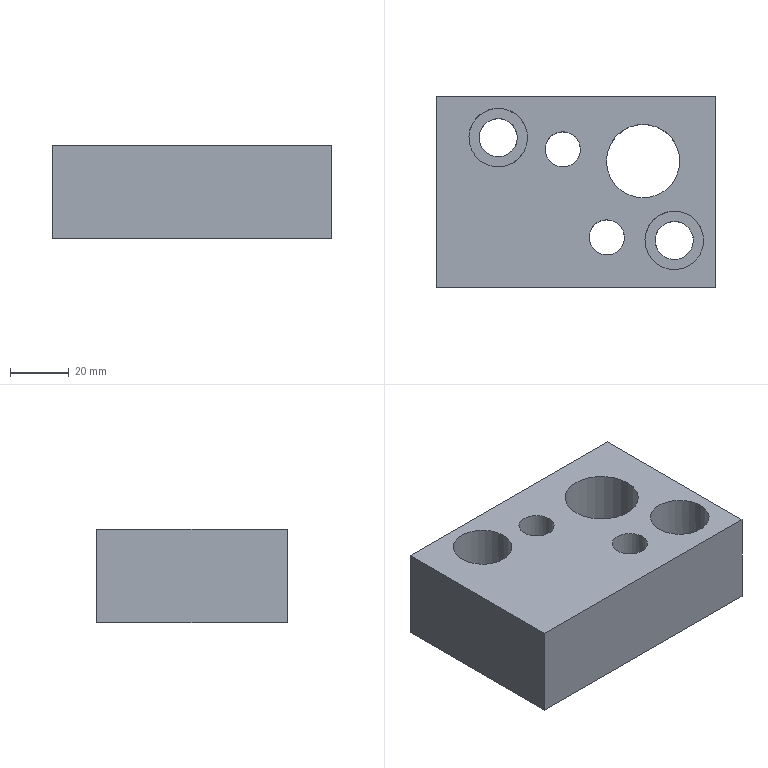Part | STEP file | gslz 2016.10.28-13_id1334_x_t | 1 solid | 17 faces | box 95 x 65 x 32 mm | volume 157873 mm3 | plane 9 | cylinder 8 | commonest cylinder face diameters 12 x2 13 x2 20 x2 25 x1 32 x1
STEP:
#1=CARTESIAN_POINT('',(0.,0.,0.));
#2=DIRECTION('',(0.,0.,1.));
#3=DIRECTION('',(1.,0.,0.));
#4=AXIS2_PLACEMENT_3D('',#1,#2,#3);
#5=CARTESIAN_POINT('',(-1412.127,66.996,-26.4));
#6=VERTEX_POINT('',#5);
#7=CARTESIAN_POINT('',(-1424.627,66.996,-26.4));
#8=DIRECTION('',(0.,0.,1.));
#9=DIRECTION('',(1.,0.,0.));
#10=AXIS2_PLACEMENT_3D('',#7,#8,#9);
#11=CIRCLE('',#10,12.5);
#12=CARTESIAN_POINT('',(-1424.627,66.996,-26.4));
#13=DIRECTION('',(0.,0.,1.));
#14=DIRECTION('',(1.,0.,0.));
#15=AXIS2_PLACEMENT_3D('',#12,#13,#14);
#16=PLANE('',#15);
#17=CARTESIAN_POINT('',(0.,0.));
#18=DIRECTION('',(1.,0.));
#19=AXIS2_PLACEMENT_2D('',#17,#18);
#20=CIRCLE('',#19,12.5);
#21=(GEOMETRIC_REPRESENTATION_CONTEXT(2)PARAMETRIC_REPRESENTATION_CONTEXT()REPRESENTATION_CONTEXT('',''));
#22=DEFINITIONAL_REPRESENTATION('',(#20),#21);
#23=PCURVE('',#16,#22);
#24=CARTESIAN_POINT('',(-1424.627,66.996,-84.));
#25=DIRECTION('',(0.,0.,1.));
#26=DIRECTION('',(1.,0.,0.));
#27=AXIS2_PLACEMENT_3D('',#24,#25,#26);
#28=CYLINDRICAL_SURFACE('',#27,12.5);
#29=CARTESIAN_POINT('',(0.,57.6));
#30=DIRECTION('',(1.,0.));
#31=VECTOR('',#30,1.);
#32=LINE('',#29,#31);
#33=(GEOMETRIC_REPRESENTATION_CONTEXT(2)PARAMETRIC_REPRESENTATION_CONTEXT()REPRESENTATION_CONTEXT('',''));
#34=DEFINITIONAL_REPRESENTATION('',(#32),#33);
#35=PCURVE('',#28,#34);
#36=SURFACE_CURVE('',#11,(#23,#35),.PCURVE_S1.);
#37=EDGE_CURVE('',#6,#6,#36,.T.);
#38=ORIENTED_EDGE('',*,*,#37,.T.);
#39=EDGE_LOOP('',(#38));
#40=FACE_BOUND('',#39,.T.);
#41=CARTESIAN_POINT('',(-1408.627,66.996,-26.4));
#42=VERTEX_POINT('',#41);
#43=CARTESIAN_POINT('',(-1424.627,66.996,-26.4));
#44=DIRECTION('',(0.,0.,-1.));
#45=DIRECTION('',(1.,0.,0.));
#46=AXIS2_PLACEMENT_3D('',#43,#44,#45);
#47=CIRCLE('',#46,16.);
#48=CARTESIAN_POINT('',(16.,0.));
#49=CARTESIAN_POINT('',(16.,-27.713));
#50=CARTESIAN_POINT('',(-8.,-13.856));
#51=CARTESIAN_POINT('',(-32.,0.));
#52=CARTESIAN_POINT('',(-8.,13.856));
#53=CARTESIAN_POINT('',(16.,27.713));
#54=CARTESIAN_POINT('',(16.,0.));
#55=(BOUNDED_CURVE()B_SPLINE_CURVE(2,(#48,#49,#50,#51,#52,#53,#54),.UNSPECIFIED.,.T.,.F.)B_SPLINE_CURVE_WITH_KNOTS((1,2,2,2,2,1),(-2.094,0.,2.094,4.189,6.283,8.378),.UNSPECIFIED.)CURVE()GEOMETRIC_REPRESENTATION_ITEM()RATIONAL_B_SPLINE_CURVE((1.,0.5,1.,0.5,1.,0.5,1.))REPRESENTATION_ITEM(''));
#56=(GEOMETRIC_REPRESENTATION_CONTEXT(2)PARAMETRIC_REPRESENTATION_CONTEXT()REPRESENTATION_CONTEXT('',''));
#57=DEFINITIONAL_REPRESENTATION('',(#55),#56);
#58=PCURVE('',#16,#57);
#59=CARTESIAN_POINT('',(-1424.627,66.996,-29.7));
#60=DIRECTION('',(0.,0.,-1.));
#61=DIRECTION('',(-1.,0.,0.));
#62=AXIS2_PLACEMENT_3D('',#59,#60,#61);
#63=CYLINDRICAL_SURFACE('',#62,16.);
#64=CARTESIAN_POINT('',(3.142,-3.3));
#65=DIRECTION('',(1.,0.));
#66=VECTOR('',#65,1.);
#67=LINE('',#64,#66);
#68=(GEOMETRIC_REPRESENTATION_CONTEXT(2)PARAMETRIC_REPRESENTATION_CONTEXT()REPRESENTATION_CONTEXT('',''));
#69=DEFINITIONAL_REPRESENTATION('',(#67),#68);
#70=PCURVE('',#63,#69);
#71=SURFACE_CURVE('',#47,(#58,#70),.PCURVE_S1.);
#72=EDGE_CURVE('',#42,#42,#71,.T.);
#73=ORIENTED_EDGE('',*,*,#72,.T.);
#74=EDGE_LOOP('',(#73));
#75=FACE_BOUND('',#74,.T.);
#76=ADVANCED_FACE('',(#40,#75),#16,.F.);
#77=CARTESIAN_POINT('',(-1400.,24.,0.));
#78=VERTEX_POINT('',#77);
#79=CARTESIAN_POINT('',(-1400.,89.,0.));
#80=VERTEX_POINT('',#79);
#81=CARTESIAN_POINT('',(-1400.,30.,0.));
#82=DIRECTION('',(0.,1.,0.));
#83=VECTOR('',#82,1.);
#84=LINE('',#81,#83);
#85=CARTESIAN_POINT('',(-1400.,30.,-35.));
#86=DIRECTION('',(1.,0.,0.));
#87=DIRECTION('',(0.,1.,0.));
#88=AXIS2_PLACEMENT_3D('',#85,#86,#87);
#89=PLANE('',#88);
#90=CARTESIAN_POINT('',(0.,35.));
#91=DIRECTION('',(1.,0.));
#92=VECTOR('',#91,1.);
#93=LINE('',#90,#92);
#94=(GEOMETRIC_REPRESENTATION_CONTEXT(2)PARAMETRIC_REPRESENTATION_CONTEXT()REPRESENTATION_CONTEXT('',''));
#95=DEFINITIONAL_REPRESENTATION('',(#93),#94);
#96=PCURVE('',#89,#95);
#97=CARTESIAN_POINT('',(-1374.,128.728,0.));
#98=DIRECTION('',(0.,0.,1.));
#99=DIRECTION('',(1.,0.,0.));
#100=AXIS2_PLACEMENT_3D('',#97,#98,#99);
#101=PLANE('',#100);
#102=CARTESIAN_POINT('',(-26.,-98.728));
#103=DIRECTION('',(0.,1.));
#104=VECTOR('',#103,1.);
#105=LINE('',#102,#104);
#106=(GEOMETRIC_REPRESENTATION_CONTEXT(2)PARAMETRIC_REPRESENTATION_CONTEXT()REPRESENTATION_CONTEXT('',''));
#107=DEFINITIONAL_REPRESENTATION('',(#105),#106);
#108=PCURVE('',#101,#107);
#109=SURFACE_CURVE('',#84,(#96,#108),.PCURVE_S1.);
#110=EDGE_CURVE('',#78,#80,#109,.T.);
#111=ORIENTED_EDGE('',*,*,#110,.F.);
#112=CARTESIAN_POINT('',(-1400.,24.,-32.));
#113=VERTEX_POINT('',#112);
#114=CARTESIAN_POINT('',(-1400.,24.,-35.));
#115=DIRECTION('',(0.,0.,1.));
#116=VECTOR('',#115,1.);
#117=LINE('',#114,#116);
#118=CARTESIAN_POINT('',(-6.,0.));
#119=DIRECTION('',(0.,1.));
#120=VECTOR('',#119,1.);
#121=LINE('',#118,#120);
#122=(GEOMETRIC_REPRESENTATION_CONTEXT(2)PARAMETRIC_REPRESENTATION_CONTEXT()REPRESENTATION_CONTEXT('',''));
#123=DEFINITIONAL_REPRESENTATION('',(#121),#122);
#124=PCURVE('',#89,#123);
#125=CARTESIAN_POINT('',(-1490.,24.,-35.));
#126=DIRECTION('',(0.,-1.,0.));
#127=DIRECTION('',(1.,0.,0.));
#128=AXIS2_PLACEMENT_3D('',#125,#126,#127);
#129=PLANE('',#128);
#130=CARTESIAN_POINT('',(90.,0.));
#131=DIRECTION('',(0.,1.));
#132=VECTOR('',#131,1.);
#133=LINE('',#130,#132);
#134=(GEOMETRIC_REPRESENTATION_CONTEXT(2)PARAMETRIC_REPRESENTATION_CONTEXT()REPRESENTATION_CONTEXT('',''));
#135=DEFINITIONAL_REPRESENTATION('',(#133),#134);
#136=PCURVE('',#129,#135);
#137=SURFACE_CURVE('',#117,(#124,#136),.PCURVE_S1.);
#138=EDGE_CURVE('',#113,#78,#137,.T.);
#139=ORIENTED_EDGE('',*,*,#138,.F.);
#140=CARTESIAN_POINT('',(-1400.,89.,-32.));
#141=VERTEX_POINT('',#140);
#142=CARTESIAN_POINT('',(-1400.,30.,-32.));
#143=DIRECTION('',(0.,1.,0.));
#144=VECTOR('',#143,1.);
#145=LINE('',#142,#144);
#146=CARTESIAN_POINT('',(0.,3.));
#147=DIRECTION('',(1.,0.));
#148=VECTOR('',#147,1.);
#149=LINE('',#146,#148);
#150=(GEOMETRIC_REPRESENTATION_CONTEXT(2)PARAMETRIC_REPRESENTATION_CONTEXT()REPRESENTATION_CONTEXT('',''));
#151=DEFINITIONAL_REPRESENTATION('',(#149),#150);
#152=PCURVE('',#89,#151);
#153=CARTESIAN_POINT('',(-1374.,128.728,-32.));
#154=DIRECTION('',(0.,0.,1.));
#155=DIRECTION('',(1.,0.,0.));
#156=AXIS2_PLACEMENT_3D('',#153,#154,#155);
#157=PLANE('',#156);
#158=CARTESIAN_POINT('',(-26.,-98.728));
#159=DIRECTION('',(0.,1.));
#160=VECTOR('',#159,1.);
#161=LINE('',#158,#160);
#162=(GEOMETRIC_REPRESENTATION_CONTEXT(2)PARAMETRIC_REPRESENTATION_CONTEXT()REPRESENTATION_CONTEXT('',''));
#163=DEFINITIONAL_REPRESENTATION('',(#161),#162);
#164=PCURVE('',#157,#163);
#165=SURFACE_CURVE('',#145,(#152,#164),.PCURVE_S1.);
#166=EDGE_CURVE('',#113,#141,#165,.T.);
#167=ORIENTED_EDGE('',*,*,#166,.T.);
#168=CARTESIAN_POINT('',(-1400.,89.,-35.));
#169=DIRECTION('',(0.,0.,-1.));
#170=VECTOR('',#169,1.);
#171=LINE('',#168,#170);
#172=CARTESIAN_POINT('',(59.,0.));
#173=DIRECTION('',(0.,-1.));
#174=VECTOR('',#173,1.);
#175=LINE('',#172,#174);
#176=(GEOMETRIC_REPRESENTATION_CONTEXT(2)PARAMETRIC_REPRESENTATION_CONTEXT()REPRESENTATION_CONTEXT('',''));
#177=DEFINITIONAL_REPRESENTATION('',(#175),#176);
#178=PCURVE('',#89,#177);
#179=CARTESIAN_POINT('',(-1445.,89.,-17.5));
#180=DIRECTION('',(0.,-1.,0.));
#181=DIRECTION('',(0.,0.,-1.));
#182=AXIS2_PLACEMENT_3D('',#179,#180,#181);
#183=PLANE('',#182);
#184=CARTESIAN_POINT('',(17.5,45.));
#185=DIRECTION('',(1.,0.));
#186=VECTOR('',#185,1.);
#187=LINE('',#184,#186);
#188=(GEOMETRIC_REPRESENTATION_CONTEXT(2)PARAMETRIC_REPRESENTATION_CONTEXT()REPRESENTATION_CONTEXT('',''));
#189=DEFINITIONAL_REPRESENTATION('',(#187),#188);
#190=PCURVE('',#183,#189);
#191=SURFACE_CURVE('',#171,(#178,#190),.PCURVE_S1.);
#192=EDGE_CURVE('',#80,#141,#191,.T.);
#193=ORIENTED_EDGE('',*,*,#192,.F.);
#194=EDGE_LOOP('',(#111,#139,#167,#193));
#195=FACE_BOUND('',#194,.T.);
#196=ADVANCED_FACE('',(#195),#89,.T.);
#197=CARTESIAN_POINT('',(-1495.,24.,0.));
#198=VERTEX_POINT('',#197);
#199=CARTESIAN_POINT('',(-1490.,24.,0.));
#200=DIRECTION('',(1.,0.,0.));
#201=VECTOR('',#200,1.);
#202=LINE('',#199,#201);
#203=CARTESIAN_POINT('',(0.,35.));
#204=DIRECTION('',(1.,0.));
#205=VECTOR('',#204,1.);
#206=LINE('',#203,#205);
#207=(GEOMETRIC_REPRESENTATION_CONTEXT(2)PARAMETRIC_REPRESENTATION_CONTEXT()REPRESENTATION_CONTEXT('',''));
#208=DEFINITIONAL_REPRESENTATION('',(#206),#207);
#209=PCURVE('',#129,#208);
#210=CARTESIAN_POINT('',(-116.,-104.728));
#211=DIRECTION('',(1.,0.));
#212=VECTOR('',#211,1.);
#213=LINE('',#210,#212);
#214=(GEOMETRIC_REPRESENTATION_CONTEXT(2)PARAMETRIC_REPRESENTATION_CONTEXT()REPRESENTATION_CONTEXT('',''));
#215=DEFINITIONAL_REPRESENTATION('',(#213),#214);
#216=PCURVE('',#101,#215);
#217=SURFACE_CURVE('',#202,(#209,#216),.PCURVE_S1.);
#218=EDGE_CURVE('',#198,#78,#217,.T.);
#219=ORIENTED_EDGE('',*,*,#218,.F.);
#220=CARTESIAN_POINT('',(-1495.,24.,-32.));
#221=VERTEX_POINT('',#220);
#222=CARTESIAN_POINT('',(-1495.,24.,-35.));
#223=DIRECTION('',(0.,0.,1.));
#224=VECTOR('',#223,1.);
#225=LINE('',#222,#224);
#226=CARTESIAN_POINT('',(-5.,0.));
#227=DIRECTION('',(0.,1.));
#228=VECTOR('',#227,1.);
#229=LINE('',#226,#228);
#230=(GEOMETRIC_REPRESENTATION_CONTEXT(2)PARAMETRIC_REPRESENTATION_CONTEXT()REPRESENTATION_CONTEXT('',''));
#231=DEFINITIONAL_REPRESENTATION('',(#229),#230);
#232=PCURVE('',#129,#231);
#233=CARTESIAN_POINT('',(-1495.,220.,-35.));
#234=DIRECTION('',(-1.,0.,0.));
#235=DIRECTION('',(0.,0.,1.));
#236=AXIS2_PLACEMENT_3D('',#233,#234,#235);
#237=PLANE('',#236);
#238=CARTESIAN_POINT('',(0.,-196.));
#239=DIRECTION('',(1.,0.));
#240=VECTOR('',#239,1.);
#241=LINE('',#238,#240);
#242=(GEOMETRIC_REPRESENTATION_CONTEXT(2)PARAMETRIC_REPRESENTATION_CONTEXT()REPRESENTATION_CONTEXT('',''));
#243=DEFINITIONAL_REPRESENTATION('',(#241),#242);
#244=PCURVE('',#237,#243);
#245=SURFACE_CURVE('',#225,(#232,#244),.PCURVE_S1.);
#246=EDGE_CURVE('',#221,#198,#245,.T.);
#247=ORIENTED_EDGE('',*,*,#246,.F.);
#248=CARTESIAN_POINT('',(-1490.,24.,-32.));
#249=DIRECTION('',(1.,0.,0.));
#250=VECTOR('',#249,1.);
#251=LINE('',#248,#250);
#252=CARTESIAN_POINT('',(0.,3.));
#253=DIRECTION('',(1.,0.));
#254=VECTOR('',#253,1.);
#255=LINE('',#252,#254);
#256=(GEOMETRIC_REPRESENTATION_CONTEXT(2)PARAMETRIC_REPRESENTATION_CONTEXT()REPRESENTATION_CONTEXT('',''));
#257=DEFINITIONAL_REPRESENTATION('',(#255),#256);
#258=PCURVE('',#129,#257);
#259=CARTESIAN_POINT('',(-116.,-104.728));
#260=DIRECTION('',(1.,0.));
#261=VECTOR('',#260,1.);
#262=LINE('',#259,#261);
#263=(GEOMETRIC_REPRESENTATION_CONTEXT(2)PARAMETRIC_REPRESENTATION_CONTEXT()REPRESENTATION_CONTEXT('',''));
#264=DEFINITIONAL_REPRESENTATION('',(#262),#263);
#265=PCURVE('',#157,#264);
#266=SURFACE_CURVE('',#251,(#258,#265),.PCURVE_S1.);
#267=EDGE_CURVE('',#221,#113,#266,.T.);
#268=ORIENTED_EDGE('',*,*,#267,.T.);
#269=ORIENTED_EDGE('',*,*,#138,.T.);
#270=EDGE_LOOP('',(#219,#247,#268,#269));
#271=FACE_BOUND('',#270,.T.);
#272=ADVANCED_FACE('',(#271),#129,.T.);
#273=CARTESIAN_POINT('',(-1495.,89.,0.));
#274=VERTEX_POINT('',#273);
#275=CARTESIAN_POINT('',(-1495.,89.,-32.));
#276=VERTEX_POINT('',#275);
#277=CARTESIAN_POINT('',(-1495.,89.,-35.));
#278=DIRECTION('',(0.,0.,-1.));
#279=VECTOR('',#278,1.);
#280=LINE('',#277,#279);
#281=CARTESIAN_POINT('',(0.,-131.));
#282=DIRECTION('',(-1.,0.));
#283=VECTOR('',#282,1.);
#284=LINE('',#281,#283);
#285=(GEOMETRIC_REPRESENTATION_CONTEXT(2)PARAMETRIC_REPRESENTATION_CONTEXT()REPRESENTATION_CONTEXT('',''));
#286=DEFINITIONAL_REPRESENTATION('',(#284),#285);
#287=PCURVE('',#237,#286);
#288=CARTESIAN_POINT('',(17.5,-50.));
#289=DIRECTION('',(1.,0.));
#290=VECTOR('',#289,1.);
#291=LINE('',#288,#290);
#292=(GEOMETRIC_REPRESENTATION_CONTEXT(2)PARAMETRIC_REPRESENTATION_CONTEXT()REPRESENTATION_CONTEXT('',''));
#293=DEFINITIONAL_REPRESENTATION('',(#291),#292);
#294=PCURVE('',#183,#293);
#295=SURFACE_CURVE('',#280,(#287,#294),.PCURVE_S1.);
#296=EDGE_CURVE('',#274,#276,#295,.T.);
#297=ORIENTED_EDGE('',*,*,#296,.T.);
#298=CARTESIAN_POINT('',(-1495.,220.,-32.));
#299=DIRECTION('',(0.,-1.,0.));
#300=VECTOR('',#299,1.);
#301=LINE('',#298,#300);
#302=CARTESIAN_POINT('',(3.,0.));
#303=DIRECTION('',(0.,-1.));
#304=VECTOR('',#303,1.);
#305=LINE('',#302,#304);
#306=(GEOMETRIC_REPRESENTATION_CONTEXT(2)PARAMETRIC_REPRESENTATION_CONTEXT()REPRESENTATION_CONTEXT('',''));
#307=DEFINITIONAL_REPRESENTATION('',(#305),#306);
#308=PCURVE('',#237,#307);
#309=CARTESIAN_POINT('',(-121.,91.272));
#310=DIRECTION('',(0.,-1.));
#311=VECTOR('',#310,1.);
#312=LINE('',#309,#311);
#313=(GEOMETRIC_REPRESENTATION_CONTEXT(2)PARAMETRIC_REPRESENTATION_CONTEXT()REPRESENTATION_CONTEXT('',''));
#314=DEFINITIONAL_REPRESENTATION('',(#312),#313);
#315=PCURVE('',#157,#314);
#316=SURFACE_CURVE('',#301,(#308,#315),.PCURVE_S1.);
#317=EDGE_CURVE('',#276,#221,#316,.T.);
#318=ORIENTED_EDGE('',*,*,#317,.T.);
#319=ORIENTED_EDGE('',*,*,#246,.T.);
#320=CARTESIAN_POINT('',(-1495.,220.,0.));
#321=DIRECTION('',(0.,-1.,0.));
#322=VECTOR('',#321,1.);
#323=LINE('',#320,#322);
#324=CARTESIAN_POINT('',(35.,0.));
#325=DIRECTION('',(0.,-1.));
#326=VECTOR('',#325,1.);
#327=LINE('',#324,#326);
#328=(GEOMETRIC_REPRESENTATION_CONTEXT(2)PARAMETRIC_REPRESENTATION_CONTEXT()REPRESENTATION_CONTEXT('',''));
#329=DEFINITIONAL_REPRESENTATION('',(#327),#328);
#330=PCURVE('',#237,#329);
#331=CARTESIAN_POINT('',(-121.,91.272));
#332=DIRECTION('',(0.,-1.));
#333=VECTOR('',#332,1.);
#334=LINE('',#331,#333);
#335=(GEOMETRIC_REPRESENTATION_CONTEXT(2)PARAMETRIC_REPRESENTATION_CONTEXT()REPRESENTATION_CONTEXT('',''));
#336=DEFINITIONAL_REPRESENTATION('',(#334),#335);
#337=PCURVE('',#101,#336);
#338=SURFACE_CURVE('',#323,(#330,#337),.PCURVE_S1.);
#339=EDGE_CURVE('',#274,#198,#338,.T.);
#340=ORIENTED_EDGE('',*,*,#339,.F.);
#341=EDGE_LOOP('',(#297,#318,#319,#340));
#342=FACE_BOUND('',#341,.T.);
#343=ADVANCED_FACE('',(#342),#237,.T.);
#344=ORIENTED_EDGE('',*,*,#296,.F.);
#345=CARTESIAN_POINT('',(-1374.,89.,0.));
#346=DIRECTION('',(1.,0.,0.));
#347=VECTOR('',#346,1.);
#348=LINE('',#345,#347);
#349=CARTESIAN_POINT('',(-17.5,71.));
#350=DIRECTION('',(0.,1.));
#351=VECTOR('',#350,1.);
#352=LINE('',#349,#351);
#353=(GEOMETRIC_REPRESENTATION_CONTEXT(2)PARAMETRIC_REPRESENTATION_CONTEXT()REPRESENTATION_CONTEXT('',''));
#354=DEFINITIONAL_REPRESENTATION('',(#352),#353);
#355=PCURVE('',#183,#354);
#356=CARTESIAN_POINT('',(0.,-39.728));
#357=DIRECTION('',(1.,0.));
#358=VECTOR('',#357,1.);
#359=LINE('',#356,#358);
#360=(GEOMETRIC_REPRESENTATION_CONTEXT(2)PARAMETRIC_REPRESENTATION_CONTEXT()REPRESENTATION_CONTEXT('',''));
#361=DEFINITIONAL_REPRESENTATION('',(#359),#360);
#362=PCURVE('',#101,#361);
#363=SURFACE_CURVE('',#348,(#355,#362),.PCURVE_S1.);
#364=EDGE_CURVE('',#274,#80,#363,.T.);
#365=ORIENTED_EDGE('',*,*,#364,.T.);
#366=ORIENTED_EDGE('',*,*,#192,.T.);
#367=CARTESIAN_POINT('',(-1374.,89.,-32.));
#368=DIRECTION('',(-1.,0.,0.));
#369=VECTOR('',#368,1.);
#370=LINE('',#367,#369);
#371=CARTESIAN_POINT('',(14.5,71.));
#372=DIRECTION('',(0.,-1.));
#373=VECTOR('',#372,1.);
#374=LINE('',#371,#373);
#375=(GEOMETRIC_REPRESENTATION_CONTEXT(2)PARAMETRIC_REPRESENTATION_CONTEXT()REPRESENTATION_CONTEXT('',''));
#376=DEFINITIONAL_REPRESENTATION('',(#374),#375);
#377=PCURVE('',#183,#376);
#378=CARTESIAN_POINT('',(0.,-39.728));
#379=DIRECTION('',(-1.,0.));
#380=VECTOR('',#379,1.);
#381=LINE('',#378,#380);
#382=(GEOMETRIC_REPRESENTATION_CONTEXT(2)PARAMETRIC_REPRESENTATION_CONTEXT()REPRESENTATION_CONTEXT('',''));
#383=DEFINITIONAL_REPRESENTATION('',(#381),#382);
#384=PCURVE('',#157,#383);
#385=SURFACE_CURVE('',#370,(#377,#384),.PCURVE_S1.);
#386=EDGE_CURVE('',#141,#276,#385,.T.);
#387=ORIENTED_EDGE('',*,*,#386,.T.);
#388=EDGE_LOOP('',(#344,#365,#366,#387));
#389=FACE_BOUND('',#388,.T.);
#390=ADVANCED_FACE('',(#389),#183,.F.);
#391=ORIENTED_EDGE('',*,*,#37,.T.);
#392=CARTESIAN_POINT('',(-1412.127,66.996,0.));
#393=VERTEX_POINT('',#392);
#394=CARTESIAN_POINT('',(-1412.127,66.996,-26.4));
#395=CARTESIAN_POINT('',(-1412.127,66.996,0.));
#396=B_SPLINE_CURVE_WITH_KNOTS('',1,(#394,#395),.UNSPECIFIED.,.F.,.F.,(2,2),(57.6,84.),.PIECEWISE_BEZIER_KNOTS.);
#397=CARTESIAN_POINT('',(6.283,0.));
#398=DIRECTION('',(0.,1.));
#399=VECTOR('',#398,1.);
#400=LINE('',#397,#399);
#401=(GEOMETRIC_REPRESENTATION_CONTEXT(2)PARAMETRIC_REPRESENTATION_CONTEXT()REPRESENTATION_CONTEXT('',''));
#402=DEFINITIONAL_REPRESENTATION('',(#400),#401);
#403=PCURVE('',#28,#402);
#404=CARTESIAN_POINT('',(0.,0.));
#405=DIRECTION('',(0.,1.));
#406=VECTOR('',#405,1.);
#407=LINE('',#404,#406);
#408=(GEOMETRIC_REPRESENTATION_CONTEXT(2)PARAMETRIC_REPRESENTATION_CONTEXT()REPRESENTATION_CONTEXT('',''));
#409=DEFINITIONAL_REPRESENTATION('',(#407),#408);
#410=PCURVE('',#28,#409);
#411=SEAM_CURVE('',#396,(#403,#410),.PCURVE_S1.);
#412=EDGE_CURVE('',#6,#393,#411,.T.);
#413=ORIENTED_EDGE('',*,*,#412,.T.);
#414=CARTESIAN_POINT('',(-1424.627,66.996,0.));
#415=DIRECTION('',(0.,0.,-1.));
#416=DIRECTION('',(1.,0.,0.));
#417=AXIS2_PLACEMENT_3D('',#414,#415,#416);
#418=CIRCLE('',#417,12.5);
#419=CARTESIAN_POINT('',(6.283,84.));
#420=DIRECTION('',(-1.,0.));
#421=VECTOR('',#420,1.);
#422=LINE('',#419,#421);
#423=(GEOMETRIC_REPRESENTATION_CONTEXT(2)PARAMETRIC_REPRESENTATION_CONTEXT()REPRESENTATION_CONTEXT('',''));
#424=DEFINITIONAL_REPRESENTATION('',(#422),#423);
#425=PCURVE('',#28,#424);
#426=CARTESIAN_POINT('',(-38.127,-61.732));
#427=CARTESIAN_POINT('',(-38.127,-83.383));
#428=CARTESIAN_POINT('',(-56.877,-72.557));
#429=CARTESIAN_POINT('',(-75.627,-61.732));
#430=CARTESIAN_POINT('',(-56.877,-50.907));
#431=CARTESIAN_POINT('',(-38.127,-40.081));
#432=CARTESIAN_POINT('',(-38.127,-61.732));
#433=(BOUNDED_CURVE()B_SPLINE_CURVE(2,(#426,#427,#428,#429,#430,#431,#432),.UNSPECIFIED.,.T.,.F.)B_SPLINE_CURVE_WITH_KNOTS((1,2,2,2,2,1),(-2.094,0.,2.094,4.189,6.283,8.378),.UNSPECIFIED.)CURVE()GEOMETRIC_REPRESENTATION_ITEM()RATIONAL_B_SPLINE_CURVE((1.,0.5,1.,0.5,1.,0.5,1.))REPRESENTATION_ITEM(''));
#434=(GEOMETRIC_REPRESENTATION_CONTEXT(2)PARAMETRIC_REPRESENTATION_CONTEXT()REPRESENTATION_CONTEXT('',''));
#435=DEFINITIONAL_REPRESENTATION('',(#433),#434);
#436=PCURVE('',#101,#435);
#437=SURFACE_CURVE('',#418,(#425,#436),.PCURVE_S1.);
#438=EDGE_CURVE('',#393,#393,#437,.T.);
#439=ORIENTED_EDGE('',*,*,#438,.T.);
#440=ORIENTED_EDGE('',*,*,#412,.F.);
#441=EDGE_LOOP('',(#391,#413,#439,#440));
#442=FACE_BOUND('',#441,.F.);
#443=ADVANCED_FACE('',(#442),#28,.F.);
#444=CARTESIAN_POINT('',(-1404.,40.,0.));
#445=VERTEX_POINT('',#444);
#446=CARTESIAN_POINT('',(-1415.678,30.142,0.));
#447=VERTEX_POINT('',#446);
#448=CARTESIAN_POINT('',(-1414.,40.,0.));
#449=DIRECTION('',(0.,0.,1.));
#450=DIRECTION('',(1.,0.,0.));
#451=AXIS2_PLACEMENT_3D('',#448,#449,#450);
#452=CIRCLE('',#451,10.);
#453=CARTESIAN_POINT('',(-40.,-88.728));
#454=DIRECTION('',(1.,0.));
#455=AXIS2_PLACEMENT_2D('',#453,#454);
#456=CIRCLE('',#455,10.);
#457=(GEOMETRIC_REPRESENTATION_CONTEXT(2)PARAMETRIC_REPRESENTATION_CONTEXT()REPRESENTATION_CONTEXT('',''));
#458=DEFINITIONAL_REPRESENTATION('',(#456),#457);
#459=PCURVE('',#101,#458);
#460=CARTESIAN_POINT('',(-1414.,40.,-0.5408));
#461=DIRECTION('',(0.,0.,-1.));
#462=DIRECTION('',(-1.,0.,0.));
#463=AXIS2_PLACEMENT_3D('',#460,#461,#462);
#464=CYLINDRICAL_SURFACE('',#463,10.);
#465=CARTESIAN_POINT('',(9.425,-0.5408));
#466=DIRECTION('',(-1.,0.));
#467=VECTOR('',#466,1.);
#468=LINE('',#465,#467);
#469=(GEOMETRIC_REPRESENTATION_CONTEXT(2)PARAMETRIC_REPRESENTATION_CONTEXT()REPRESENTATION_CONTEXT('',''));
#470=DEFINITIONAL_REPRESENTATION('',(#468),#469);
#471=PCURVE('',#464,#470);
#472=SURFACE_CURVE('',#452,(#459,#471),.PCURVE_S1.);
#473=EDGE_CURVE('',#445,#447,#472,.T.);
#474=ORIENTED_EDGE('',*,*,#473,.F.);
#475=CARTESIAN_POINT('',(-1414.,40.,0.));
#476=DIRECTION('',(0.,0.,1.));
#477=DIRECTION('',(1.,0.,0.));
#478=AXIS2_PLACEMENT_3D('',#475,#476,#477);
#479=CIRCLE('',#478,10.);
#480=CARTESIAN_POINT('',(-40.,-88.728));
#481=DIRECTION('',(1.,0.));
#482=AXIS2_PLACEMENT_2D('',#480,#481);
#483=CIRCLE('',#482,10.);
#484=(GEOMETRIC_REPRESENTATION_CONTEXT(2)PARAMETRIC_REPRESENTATION_CONTEXT()REPRESENTATION_CONTEXT('',''));
#485=DEFINITIONAL_REPRESENTATION('',(#483),#484);
#486=PCURVE('',#101,#485);
#487=CARTESIAN_POINT('',(15.708,-0.5408));
#488=DIRECTION('',(-1.,0.));
#489=VECTOR('',#488,1.);
#490=LINE('',#487,#489);
#491=(GEOMETRIC_REPRESENTATION_CONTEXT(2)PARAMETRIC_REPRESENTATION_CONTEXT()REPRESENTATION_CONTEXT('',''));
#492=DEFINITIONAL_REPRESENTATION('',(#490),#491);
#493=PCURVE('',#464,#492);
#494=SURFACE_CURVE('',#479,(#486,#493),.PCURVE_S1.);
#495=EDGE_CURVE('',#447,#445,#494,.T.);
#496=ORIENTED_EDGE('',*,*,#495,.F.);
#497=EDGE_LOOP('',(#474,#496));
#498=FACE_BOUND('',#497,.T.);
#499=CARTESIAN_POINT('',(-1431.,41.,0.));
#500=VERTEX_POINT('',#499);
#501=CARTESIAN_POINT('',(-1435.679,46.853,0.));
#502=VERTEX_POINT('',#501);
#503=CARTESIAN_POINT('',(-1437.,41.,0.));
#504=DIRECTION('',(0.,0.,1.));
#505=DIRECTION('',(1.,0.,0.));
#506=AXIS2_PLACEMENT_3D('',#503,#504,#505);
#507=CIRCLE('',#506,6.);
#508=CARTESIAN_POINT('',(-63.,-87.728));
#509=DIRECTION('',(1.,0.));
#510=AXIS2_PLACEMENT_2D('',#508,#509);
#511=CIRCLE('',#510,6.);
#512=(GEOMETRIC_REPRESENTATION_CONTEXT(2)PARAMETRIC_REPRESENTATION_CONTEXT()REPRESENTATION_CONTEXT('',''));
#513=DEFINITIONAL_REPRESENTATION('',(#511),#512);
#514=PCURVE('',#101,#513);
#515=CARTESIAN_POINT('',(-1437.,41.,-9.));
#516=DIRECTION('',(0.,0.,-1.));
#517=DIRECTION('',(-1.,0.,0.));
#518=AXIS2_PLACEMENT_3D('',#515,#516,#517);
#519=CYLINDRICAL_SURFACE('',#518,6.);
#520=CARTESIAN_POINT('',(3.142,-9.));
#521=DIRECTION('',(-1.,0.));
#522=VECTOR('',#521,1.);
#523=LINE('',#520,#522);
#524=(GEOMETRIC_REPRESENTATION_CONTEXT(2)PARAMETRIC_REPRESENTATION_CONTEXT()REPRESENTATION_CONTEXT('',''));
#525=DEFINITIONAL_REPRESENTATION('',(#523),#524);
#526=PCURVE('',#519,#525);
#527=SURFACE_CURVE('',#507,(#514,#526),.PCURVE_S1.);
#528=EDGE_CURVE('',#500,#502,#527,.T.);
#529=ORIENTED_EDGE('',*,*,#528,.F.);
#530=CARTESIAN_POINT('',(-1437.,41.,0.));
#531=DIRECTION('',(0.,0.,1.));
#532=DIRECTION('',(1.,0.,0.));
#533=AXIS2_PLACEMENT_3D('',#530,#531,#532);
#534=CIRCLE('',#533,6.);
#535=CARTESIAN_POINT('',(-63.,-87.728));
#536=DIRECTION('',(1.,0.));
#537=AXIS2_PLACEMENT_2D('',#535,#536);
#538=CIRCLE('',#537,6.);
#539=(GEOMETRIC_REPRESENTATION_CONTEXT(2)PARAMETRIC_REPRESENTATION_CONTEXT()REPRESENTATION_CONTEXT('',''));
#540=DEFINITIONAL_REPRESENTATION('',(#538),#539);
#541=PCURVE('',#101,#540);
#542=CARTESIAN_POINT('',(9.425,-9.));
#543=DIRECTION('',(-1.,0.));
#544=VECTOR('',#543,1.);
#545=LINE('',#542,#544);
#546=(GEOMETRIC_REPRESENTATION_CONTEXT(2)PARAMETRIC_REPRESENTATION_CONTEXT()REPRESENTATION_CONTEXT('',''));
#547=DEFINITIONAL_REPRESENTATION('',(#545),#546);
#548=PCURVE('',#519,#547);
#549=SURFACE_CURVE('',#534,(#541,#548),.PCURVE_S1.);
#550=EDGE_CURVE('',#502,#500,#549,.T.);
#551=ORIENTED_EDGE('',*,*,#550,.F.);
#552=EDGE_LOOP('',(#529,#551));
#553=FACE_BOUND('',#552,.T.);
#554=CARTESIAN_POINT('',(-1446.,71.,0.));
#555=VERTEX_POINT('',#554);
#556=CARTESIAN_POINT('',(-1450.679,76.853,0.));
#557=VERTEX_POINT('',#556);
#558=CARTESIAN_POINT('',(-1452.,71.,0.));
#559=DIRECTION('',(0.,0.,1.));
#560=DIRECTION('',(1.,0.,0.));
#561=AXIS2_PLACEMENT_3D('',#558,#559,#560);
#562=CIRCLE('',#561,6.);
#563=CARTESIAN_POINT('',(-78.,-57.728));
#564=DIRECTION('',(1.,0.));
#565=AXIS2_PLACEMENT_2D('',#563,#564);
#566=CIRCLE('',#565,6.);
#567=(GEOMETRIC_REPRESENTATION_CONTEXT(2)PARAMETRIC_REPRESENTATION_CONTEXT()REPRESENTATION_CONTEXT('',''));
#568=DEFINITIONAL_REPRESENTATION('',(#566),#567);
#569=PCURVE('',#101,#568);
#570=CARTESIAN_POINT('',(-1452.,71.,-9.));
#571=DIRECTION('',(0.,0.,-1.));
#572=DIRECTION('',(-1.,0.,0.));
#573=AXIS2_PLACEMENT_3D('',#570,#571,#572);
#574=CYLINDRICAL_SURFACE('',#573,6.);
#575=CARTESIAN_POINT('',(3.142,-9.));
#576=DIRECTION('',(-1.,0.));
#577=VECTOR('',#576,1.);
#578=LINE('',#575,#577);
#579=(GEOMETRIC_REPRESENTATION_CONTEXT(2)PARAMETRIC_REPRESENTATION_CONTEXT()REPRESENTATION_CONTEXT('',''));
#580=DEFINITIONAL_REPRESENTATION('',(#578),#579);
#581=PCURVE('',#574,#580);
#582=SURFACE_CURVE('',#562,(#569,#581),.PCURVE_S1.);
#583=EDGE_CURVE('',#555,#557,#582,.T.);
#584=ORIENTED_EDGE('',*,*,#583,.F.);
#585=CARTESIAN_POINT('',(-1452.,71.,0.));
#586=DIRECTION('',(0.,0.,1.));
#587=DIRECTION('',(1.,0.,0.));
#588=AXIS2_PLACEMENT_3D('',#585,#586,#587);
#589=CIRCLE('',#588,6.);
#590=CARTESIAN_POINT('',(-78.,-57.728));
#591=DIRECTION('',(1.,0.));
#592=AXIS2_PLACEMENT_2D('',#590,#591);
#593=CIRCLE('',#592,6.);
#594=(GEOMETRIC_REPRESENTATION_CONTEXT(2)PARAMETRIC_REPRESENTATION_CONTEXT()REPRESENTATION_CONTEXT('',''));
#595=DEFINITIONAL_REPRESENTATION('',(#593),#594);
#596=PCURVE('',#101,#595);
#597=CARTESIAN_POINT('',(9.425,-9.));
#598=DIRECTION('',(-1.,0.));
#599=VECTOR('',#598,1.);
#600=LINE('',#597,#599);
#601=(GEOMETRIC_REPRESENTATION_CONTEXT(2)PARAMETRIC_REPRESENTATION_CONTEXT()REPRESENTATION_CONTEXT('',''));
#602=DEFINITIONAL_REPRESENTATION('',(#600),#601);
#603=PCURVE('',#574,#602);
#604=SURFACE_CURVE('',#589,(#596,#603),.PCURVE_S1.);
#605=EDGE_CURVE('',#557,#555,#604,.T.);
#606=ORIENTED_EDGE('',*,*,#605,.F.);
#607=EDGE_LOOP('',(#584,#606));
#608=FACE_BOUND('',#607,.T.);
#609=CARTESIAN_POINT('',(-1464.,75.,0.));
#610=VERTEX_POINT('',#609);
#611=CARTESIAN_POINT('',(-1475.678,65.142,0.));
#612=VERTEX_POINT('',#611);
#613=CARTESIAN_POINT('',(-1474.,75.,0.));
#614=DIRECTION('',(0.,0.,1.));
#615=DIRECTION('',(1.,0.,0.));
#616=AXIS2_PLACEMENT_3D('',#613,#614,#615);
#617=CIRCLE('',#616,10.);
#618=CARTESIAN_POINT('',(-100.,-53.728));
#619=DIRECTION('',(1.,0.));
#620=AXIS2_PLACEMENT_2D('',#618,#619);
#621=CIRCLE('',#620,10.);
#622=(GEOMETRIC_REPRESENTATION_CONTEXT(2)PARAMETRIC_REPRESENTATION_CONTEXT()REPRESENTATION_CONTEXT('',''));
#623=DEFINITIONAL_REPRESENTATION('',(#621),#622);
#624=PCURVE('',#101,#623);
#625=CARTESIAN_POINT('',(-1474.,75.,-0.5408));
#626=DIRECTION('',(0.,0.,-1.));
#627=DIRECTION('',(-1.,0.,0.));
#628=AXIS2_PLACEMENT_3D('',#625,#626,#627);
#629=CYLINDRICAL_SURFACE('',#628,10.);
#630=CARTESIAN_POINT('',(9.425,-0.5408));
#631=DIRECTION('',(-1.,0.));
#632=VECTOR('',#631,1.);
#633=LINE('',#630,#632);
#634=(GEOMETRIC_REPRESENTATION_CONTEXT(2)PARAMETRIC_REPRESENTATION_CONTEXT()REPRESENTATION_CONTEXT('',''));
#635=DEFINITIONAL_REPRESENTATION('',(#633),#634);
#636=PCURVE('',#629,#635);
#637=SURFACE_CURVE('',#617,(#624,#636),.PCURVE_S1.);
#638=EDGE_CURVE('',#610,#612,#637,.T.);
#639=ORIENTED_EDGE('',*,*,#638,.F.);
#640=CARTESIAN_POINT('',(-1474.,75.,0.));
#641=DIRECTION('',(0.,0.,1.));
#642=DIRECTION('',(1.,0.,0.));
#643=AXIS2_PLACEMENT_3D('',#640,#641,#642);
#644=CIRCLE('',#643,10.);
#645=CARTESIAN_POINT('',(-100.,-53.728));
#646=DIRECTION('',(1.,0.));
#647=AXIS2_PLACEMENT_2D('',#645,#646);
#648=CIRCLE('',#647,10.);
#649=(GEOMETRIC_REPRESENTATION_CONTEXT(2)PARAMETRIC_REPRESENTATION_CONTEXT()REPRESENTATION_CONTEXT('',''));
#650=DEFINITIONAL_REPRESENTATION('',(#648),#649);
#651=PCURVE('',#101,#650);
#652=CARTESIAN_POINT('',(15.708,-0.5408));
#653=DIRECTION('',(-1.,0.));
#654=VECTOR('',#653,1.);
#655=LINE('',#652,#654);
#656=(GEOMETRIC_REPRESENTATION_CONTEXT(2)PARAMETRIC_REPRESENTATION_CONTEXT()REPRESENTATION_CONTEXT('',''));
#657=DEFINITIONAL_REPRESENTATION('',(#655),#656);
#658=PCURVE('',#629,#657);
#659=SURFACE_CURVE('',#644,(#651,#658),.PCURVE_S1.);
#660=EDGE_CURVE('',#612,#610,#659,.T.);
#661=ORIENTED_EDGE('',*,*,#660,.F.);
#662=EDGE_LOOP('',(#639,#661));
#663=FACE_BOUND('',#662,.T.);
#664=ORIENTED_EDGE('',*,*,#438,.T.);
#665=EDGE_LOOP('',(#664));
#666=FACE_BOUND('',#665,.T.);
#667=ORIENTED_EDGE('',*,*,#364,.F.);
#668=ORIENTED_EDGE('',*,*,#339,.T.);
#669=ORIENTED_EDGE('',*,*,#218,.T.);
#670=ORIENTED_EDGE('',*,*,#110,.T.);
#671=EDGE_LOOP('',(#667,#668,#669,#670));
#672=FACE_BOUND('',#671,.T.);
#673=ADVANCED_FACE('',(#498,#553,#608,#663,#666,#672),#101,.T.);
#674=CARTESIAN_POINT('',(-1408.627,66.996,-32.));
#675=VERTEX_POINT('',#674);
#676=CARTESIAN_POINT('',(-1424.627,66.996,-32.));
#677=DIRECTION('',(0.,0.,1.));
#678=DIRECTION('',(1.,0.,0.));
#679=AXIS2_PLACEMENT_3D('',#676,#677,#678);
#680=CIRCLE('',#679,16.);
#681=CARTESIAN_POINT('',(9.425,2.3));
#682=DIRECTION('',(-1.,0.));
#683=VECTOR('',#682,1.);
#684=LINE('',#681,#683);
#685=(GEOMETRIC_REPRESENTATION_CONTEXT(2)PARAMETRIC_REPRESENTATION_CONTEXT()REPRESENTATION_CONTEXT('',''));
#686=DEFINITIONAL_REPRESENTATION('',(#684),#685);
#687=PCURVE('',#63,#686);
#688=CARTESIAN_POINT('',(-50.627,-61.732));
#689=DIRECTION('',(1.,0.));
#690=AXIS2_PLACEMENT_2D('',#688,#689);
#691=CIRCLE('',#690,16.);
#692=(GEOMETRIC_REPRESENTATION_CONTEXT(2)PARAMETRIC_REPRESENTATION_CONTEXT()REPRESENTATION_CONTEXT('',''));
#693=DEFINITIONAL_REPRESENTATION('',(#691),#692);
#694=PCURVE('',#157,#693);
#695=SURFACE_CURVE('',#680,(#687,#694),.PCURVE_S1.);
#696=EDGE_CURVE('',#675,#675,#695,.T.);
#697=ORIENTED_EDGE('',*,*,#696,.T.);
#698=CARTESIAN_POINT('',(-1408.627,66.996,-26.4));
#699=CARTESIAN_POINT('',(-1408.627,66.996,-32.));
#700=B_SPLINE_CURVE_WITH_KNOTS('',1,(#698,#699),.UNSPECIFIED.,.F.,.F.,(2,2),(-3.3,2.3),.PIECEWISE_BEZIER_KNOTS.);
#701=CARTESIAN_POINT('',(3.142,0.));
#702=DIRECTION('',(0.,1.));
#703=VECTOR('',#702,1.);
#704=LINE('',#701,#703);
#705=(GEOMETRIC_REPRESENTATION_CONTEXT(2)PARAMETRIC_REPRESENTATION_CONTEXT()REPRESENTATION_CONTEXT('',''));
#706=DEFINITIONAL_REPRESENTATION('',(#704),#705);
#707=PCURVE('',#63,#706);
#708=CARTESIAN_POINT('',(9.425,0.));
#709=DIRECTION('',(0.,1.));
#710=VECTOR('',#709,1.);
#711=LINE('',#708,#710);
#712=(GEOMETRIC_REPRESENTATION_CONTEXT(2)PARAMETRIC_REPRESENTATION_CONTEXT()REPRESENTATION_CONTEXT('',''));
#713=DEFINITIONAL_REPRESENTATION('',(#711),#712);
#714=PCURVE('',#63,#713);
#715=SEAM_CURVE('',#700,(#707,#714),.PCURVE_S1.);
#716=EDGE_CURVE('',#42,#675,#715,.T.);
#717=ORIENTED_EDGE('',*,*,#716,.F.);
#718=ORIENTED_EDGE('',*,*,#72,.T.);
#719=ORIENTED_EDGE('',*,*,#716,.T.);
#720=EDGE_LOOP('',(#697,#717,#718,#719));
#721=FACE_BOUND('',#720,.F.);
#722=ADVANCED_FACE('',(#721),#63,.F.);
#723=CARTESIAN_POINT('',(-1407.5,40.,-32.));
#724=VERTEX_POINT('',#723);
#725=CARTESIAN_POINT('',(-1415.091,33.592,-32.));
#726=VERTEX_POINT('',#725);
#727=CARTESIAN_POINT('',(-1414.,40.,-32.));
#728=DIRECTION('',(0.,0.,1.));
#729=DIRECTION('',(1.,0.,0.));
#730=AXIS2_PLACEMENT_3D('',#727,#728,#729);
#731=CIRCLE('',#730,6.5);
#732=CARTESIAN_POINT('',(-40.,-88.728));
#733=DIRECTION('',(1.,0.));
#734=AXIS2_PLACEMENT_2D('',#732,#733);
#735=CIRCLE('',#734,6.5);
#736=(GEOMETRIC_REPRESENTATION_CONTEXT(2)PARAMETRIC_REPRESENTATION_CONTEXT()REPRESENTATION_CONTEXT('',''));
#737=DEFINITIONAL_REPRESENTATION('',(#735),#736);
#738=PCURVE('',#157,#737);
#739=CARTESIAN_POINT('',(-1414.,40.,-0.5408));
#740=DIRECTION('',(0.,0.,-1.));
#741=DIRECTION('',(-1.,0.,0.));
#742=AXIS2_PLACEMENT_3D('',#739,#740,#741);
#743=CYLINDRICAL_SURFACE('',#742,6.5);
#744=CARTESIAN_POINT('',(9.425,31.459));
#745=DIRECTION('',(-1.,0.));
#746=VECTOR('',#745,1.);
#747=LINE('',#744,#746);
#748=(GEOMETRIC_REPRESENTATION_CONTEXT(2)PARAMETRIC_REPRESENTATION_CONTEXT()REPRESENTATION_CONTEXT('',''));
#749=DEFINITIONAL_REPRESENTATION('',(#747),#748);
#750=PCURVE('',#743,#749);
#751=SURFACE_CURVE('',#731,(#738,#750),.PCURVE_S1.);
#752=EDGE_CURVE('',#724,#726,#751,.T.);
#753=ORIENTED_EDGE('',*,*,#752,.T.);
#754=CARTESIAN_POINT('',(-1414.,40.,-32.));
#755=DIRECTION('',(0.,0.,1.));
#756=DIRECTION('',(1.,0.,0.));
#757=AXIS2_PLACEMENT_3D('',#754,#755,#756);
#758=CIRCLE('',#757,6.5);
#759=CARTESIAN_POINT('',(-40.,-88.728));
#760=DIRECTION('',(1.,0.));
#761=AXIS2_PLACEMENT_2D('',#759,#760);
#762=CIRCLE('',#761,6.5);
#763=(GEOMETRIC_REPRESENTATION_CONTEXT(2)PARAMETRIC_REPRESENTATION_CONTEXT()REPRESENTATION_CONTEXT('',''));
#764=DEFINITIONAL_REPRESENTATION('',(#762),#763);
#765=PCURVE('',#157,#764);
#766=CARTESIAN_POINT('',(15.708,31.459));
#767=DIRECTION('',(-1.,0.));
#768=VECTOR('',#767,1.);
#769=LINE('',#766,#768);
#770=(GEOMETRIC_REPRESENTATION_CONTEXT(2)PARAMETRIC_REPRESENTATION_CONTEXT()REPRESENTATION_CONTEXT('',''));
#771=DEFINITIONAL_REPRESENTATION('',(#769),#770);
#772=PCURVE('',#743,#771);
#773=SURFACE_CURVE('',#758,(#765,#772),.PCURVE_S1.);
#774=EDGE_CURVE('',#726,#724,#773,.T.);
#775=ORIENTED_EDGE('',*,*,#774,.T.);
#776=EDGE_LOOP('',(#753,#775));
#777=FACE_BOUND('',#776,.T.);
#778=CARTESIAN_POINT('',(-1435.679,46.853,-32.));
#779=VERTEX_POINT('',#778);
#780=CARTESIAN_POINT('',(-1437.,41.,-32.));
#781=DIRECTION('',(0.,0.,1.));
#782=DIRECTION('',(0.2202,0.9754,0.));
#783=AXIS2_PLACEMENT_3D('',#780,#781,#782);
#784=CIRCLE('',#783,6.);
#785=CARTESIAN_POINT('',(-63.,-87.728));
#786=DIRECTION('',(0.2202,0.9754));
#787=AXIS2_PLACEMENT_2D('',#785,#786);
#788=CIRCLE('',#787,6.);
#789=(GEOMETRIC_REPRESENTATION_CONTEXT(2)PARAMETRIC_REPRESENTATION_CONTEXT()REPRESENTATION_CONTEXT('',''));
#790=DEFINITIONAL_REPRESENTATION('',(#788),#789);
#791=PCURVE('',#157,#790);
#792=CARTESIAN_POINT('',(8.076,23.));
#793=DIRECTION('',(-1.,0.));
#794=VECTOR('',#793,1.);
#795=LINE('',#792,#794);
#796=(GEOMETRIC_REPRESENTATION_CONTEXT(2)PARAMETRIC_REPRESENTATION_CONTEXT()REPRESENTATION_CONTEXT('',''));
#797=DEFINITIONAL_REPRESENTATION('',(#795),#796);
#798=PCURVE('',#519,#797);
#799=SURFACE_CURVE('',#784,(#791,#798),.PCURVE_S1.);
#800=EDGE_CURVE('',#779,#779,#799,.T.);
#801=ORIENTED_EDGE('',*,*,#800,.T.);
#802=EDGE_LOOP('',(#801));
#803=FACE_BOUND('',#802,.T.);
#804=CARTESIAN_POINT('',(-1467.5,75.,-32.));
#805=VERTEX_POINT('',#804);
#806=CARTESIAN_POINT('',(-1475.091,68.592,-32.));
#807=VERTEX_POINT('',#806);
#808=CARTESIAN_POINT('',(-1474.,75.,-32.));
#809=DIRECTION('',(0.,0.,1.));
#810=DIRECTION('',(1.,0.,0.));
#811=AXIS2_PLACEMENT_3D('',#808,#809,#810);
#812=CIRCLE('',#811,6.5);
#813=CARTESIAN_POINT('',(-100.,-53.728));
#814=DIRECTION('',(1.,0.));
#815=AXIS2_PLACEMENT_2D('',#813,#814);
#816=CIRCLE('',#815,6.5);
#817=(GEOMETRIC_REPRESENTATION_CONTEXT(2)PARAMETRIC_REPRESENTATION_CONTEXT()REPRESENTATION_CONTEXT('',''));
#818=DEFINITIONAL_REPRESENTATION('',(#816),#817);
#819=PCURVE('',#157,#818);
#820=CARTESIAN_POINT('',(-1474.,75.,-0.5408));
#821=DIRECTION('',(0.,0.,-1.));
#822=DIRECTION('',(-1.,0.,0.));
#823=AXIS2_PLACEMENT_3D('',#820,#821,#822);
#824=CYLINDRICAL_SURFACE('',#823,6.5);
#825=CARTESIAN_POINT('',(9.425,31.459));
#826=DIRECTION('',(-1.,0.));
#827=VECTOR('',#826,1.);
#828=LINE('',#825,#827);
#829=(GEOMETRIC_REPRESENTATION_CONTEXT(2)PARAMETRIC_REPRESENTATION_CONTEXT()REPRESENTATION_CONTEXT('',''));
#830=DEFINITIONAL_REPRESENTATION('',(#828),#829);
#831=PCURVE('',#824,#830);
#832=SURFACE_CURVE('',#812,(#819,#831),.PCURVE_S1.);
#833=EDGE_CURVE('',#805,#807,#832,.T.);
#834=ORIENTED_EDGE('',*,*,#833,.T.);
#835=CARTESIAN_POINT('',(-1474.,75.,-32.));
#836=DIRECTION('',(0.,0.,1.));
#837=DIRECTION('',(1.,0.,0.));
#838=AXIS2_PLACEMENT_3D('',#835,#836,#837);
#839=CIRCLE('',#838,6.5);
#840=CARTESIAN_POINT('',(-100.,-53.728));
#841=DIRECTION('',(1.,0.));
#842=AXIS2_PLACEMENT_2D('',#840,#841);
#843=CIRCLE('',#842,6.5);
#844=(GEOMETRIC_REPRESENTATION_CONTEXT(2)PARAMETRIC_REPRESENTATION_CONTEXT()REPRESENTATION_CONTEXT('',''));
#845=DEFINITIONAL_REPRESENTATION('',(#843),#844);
#846=PCURVE('',#157,#845);
#847=CARTESIAN_POINT('',(15.708,31.459));
#848=DIRECTION('',(-1.,0.));
#849=VECTOR('',#848,1.);
#850=LINE('',#847,#849);
#851=(GEOMETRIC_REPRESENTATION_CONTEXT(2)PARAMETRIC_REPRESENTATION_CONTEXT()REPRESENTATION_CONTEXT('',''));
#852=DEFINITIONAL_REPRESENTATION('',(#850),#851);
#853=PCURVE('',#824,#852);
#854=SURFACE_CURVE('',#839,(#846,#853),.PCURVE_S1.);
#855=EDGE_CURVE('',#807,#805,#854,.T.);
#856=ORIENTED_EDGE('',*,*,#855,.T.);
#857=EDGE_LOOP('',(#834,#856));
#858=FACE_BOUND('',#857,.T.);
#859=ORIENTED_EDGE('',*,*,#696,.T.);
#860=EDGE_LOOP('',(#859));
#861=FACE_BOUND('',#860,.T.);
#862=ORIENTED_EDGE('',*,*,#317,.F.);
#863=ORIENTED_EDGE('',*,*,#386,.F.);
#864=ORIENTED_EDGE('',*,*,#166,.F.);
#865=ORIENTED_EDGE('',*,*,#267,.F.);
#866=EDGE_LOOP('',(#862,#863,#864,#865));
#867=FACE_BOUND('',#866,.T.);
#868=CARTESIAN_POINT('',(-1450.679,76.853,-32.));
#869=VERTEX_POINT('',#868);
#870=CARTESIAN_POINT('',(-1452.,71.,-32.));
#871=DIRECTION('',(0.,0.,1.));
#872=DIRECTION('',(0.2202,0.9754,0.));
#873=AXIS2_PLACEMENT_3D('',#870,#871,#872);
#874=CIRCLE('',#873,6.);
#875=CARTESIAN_POINT('',(-78.,-57.728));
#876=DIRECTION('',(0.2202,0.9754));
#877=AXIS2_PLACEMENT_2D('',#875,#876);
#878=CIRCLE('',#877,6.);
#879=(GEOMETRIC_REPRESENTATION_CONTEXT(2)PARAMETRIC_REPRESENTATION_CONTEXT()REPRESENTATION_CONTEXT('',''));
#880=DEFINITIONAL_REPRESENTATION('',(#878),#879);
#881=PCURVE('',#157,#880);
#882=CARTESIAN_POINT('',(8.076,23.));
#883=DIRECTION('',(-1.,0.));
#884=VECTOR('',#883,1.);
#885=LINE('',#882,#884);
#886=(GEOMETRIC_REPRESENTATION_CONTEXT(2)PARAMETRIC_REPRESENTATION_CONTEXT()REPRESENTATION_CONTEXT('',''));
#887=DEFINITIONAL_REPRESENTATION('',(#885),#886);
#888=PCURVE('',#574,#887);
#889=SURFACE_CURVE('',#874,(#881,#888),.PCURVE_S1.);
#890=EDGE_CURVE('',#869,#869,#889,.T.);
#891=ORIENTED_EDGE('',*,*,#890,.T.);
#892=EDGE_LOOP('',(#891));
#893=FACE_BOUND('',#892,.T.);
#894=ADVANCED_FACE('',(#777,#803,#858,#861,#867,#893),#157,.F.);
#895=CARTESIAN_POINT('',(-1475.091,68.592,-18.));
#896=VERTEX_POINT('',#895);
#897=CARTESIAN_POINT('',(-1474.,75.,-18.));
#898=DIRECTION('',(0.,0.,1.));
#899=DIRECTION('',(-0.1678,-0.9858,0.));
#900=AXIS2_PLACEMENT_3D('',#897,#898,#899);
#901=CIRCLE('',#900,6.5);
#902=CARTESIAN_POINT('',(11.164,17.459));
#903=DIRECTION('',(-1.,0.));
#904=VECTOR('',#903,1.);
#905=LINE('',#902,#904);
#906=(GEOMETRIC_REPRESENTATION_CONTEXT(2)PARAMETRIC_REPRESENTATION_CONTEXT()REPRESENTATION_CONTEXT('',''));
#907=DEFINITIONAL_REPRESENTATION('',(#905),#906);
#908=PCURVE('',#824,#907);
#909=CARTESIAN_POINT('',(-1474.,75.,-18.));
#910=DIRECTION('',(0.,0.,1.));
#911=DIRECTION('',(-0.1678,-0.9858,0.));
#912=AXIS2_PLACEMENT_3D('',#909,#910,#911);
#913=PLANE('',#912);
#914=CARTESIAN_POINT('',(0.,0.));
#915=DIRECTION('',(1.,0.));
#916=AXIS2_PLACEMENT_2D('',#914,#915);
#917=CIRCLE('',#916,6.5);
#918=(GEOMETRIC_REPRESENTATION_CONTEXT(2)PARAMETRIC_REPRESENTATION_CONTEXT()REPRESENTATION_CONTEXT('',''));
#919=DEFINITIONAL_REPRESENTATION('',(#917),#918);
#920=PCURVE('',#913,#919);
#921=SURFACE_CURVE('',#901,(#908,#920),.PCURVE_S1.);
#922=EDGE_CURVE('',#896,#896,#921,.T.);
#923=ORIENTED_EDGE('',*,*,#922,.F.);
#924=CARTESIAN_POINT('',(-1475.091,68.592,-18.));
#925=CARTESIAN_POINT('',(-1475.091,68.592,-32.));
#926=B_SPLINE_CURVE_WITH_KNOTS('',1,(#924,#925),.UNSPECIFIED.,.F.,.F.,(2,2),(17.459,31.459),.PIECEWISE_BEZIER_KNOTS.);
#927=CARTESIAN_POINT('',(11.164,0.));
#928=DIRECTION('',(0.,1.));
#929=VECTOR('',#928,1.);
#930=LINE('',#927,#929);
#931=(GEOMETRIC_REPRESENTATION_CONTEXT(2)PARAMETRIC_REPRESENTATION_CONTEXT()REPRESENTATION_CONTEXT('',''));
#932=DEFINITIONAL_REPRESENTATION('',(#930),#931);
#933=PCURVE('',#824,#932);
#934=CARTESIAN_POINT('',(4.881,0.));
#935=DIRECTION('',(0.,1.));
#936=VECTOR('',#935,1.);
#937=LINE('',#934,#936);
#938=(GEOMETRIC_REPRESENTATION_CONTEXT(2)PARAMETRIC_REPRESENTATION_CONTEXT()REPRESENTATION_CONTEXT('',''));
#939=DEFINITIONAL_REPRESENTATION('',(#937),#938);
#940=PCURVE('',#824,#939);
#941=SEAM_CURVE('',#926,(#933,#940),.PCURVE_S1.);
#942=EDGE_CURVE('',#896,#807,#941,.T.);
#943=ORIENTED_EDGE('',*,*,#942,.T.);
#944=ORIENTED_EDGE('',*,*,#855,.T.);
#945=ORIENTED_EDGE('',*,*,#833,.T.);
#946=ORIENTED_EDGE('',*,*,#942,.F.);
#947=EDGE_LOOP('',(#923,#943,#944,#945,#946));
#948=FACE_BOUND('',#947,.F.);
#949=ADVANCED_FACE('',(#948),#824,.F.);
#950=ORIENTED_EDGE('',*,*,#922,.F.);
#951=EDGE_LOOP('',(#950));
#952=FACE_BOUND('',#951,.T.);
#953=CARTESIAN_POINT('',(-1475.678,65.142,-18.));
#954=VERTEX_POINT('',#953);
#955=CARTESIAN_POINT('',(-1474.,75.,-18.));
#956=DIRECTION('',(0.,0.,-1.));
#957=DIRECTION('',(-0.1678,-0.9858,0.));
#958=AXIS2_PLACEMENT_3D('',#955,#956,#957);
#959=CIRCLE('',#958,10.);
#960=CARTESIAN_POINT('',(10.,0.));
#961=CARTESIAN_POINT('',(10.,-17.321));
#962=CARTESIAN_POINT('',(-5.,-8.66));
#963=CARTESIAN_POINT('',(-20.,0.));
#964=CARTESIAN_POINT('',(-5.,8.66));
#965=CARTESIAN_POINT('',(10.,17.321));
#966=CARTESIAN_POINT('',(10.,0.));
#967=(BOUNDED_CURVE()B_SPLINE_CURVE(2,(#960,#961,#962,#963,#964,#965,#966),.UNSPECIFIED.,.T.,.F.)B_SPLINE_CURVE_WITH_KNOTS((1,2,2,2,2,1),(-2.094,0.,2.094,4.189,6.283,8.378),.UNSPECIFIED.)CURVE()GEOMETRIC_REPRESENTATION_ITEM()RATIONAL_B_SPLINE_CURVE((1.,0.5,1.,0.5,1.,0.5,1.))REPRESENTATION_ITEM(''));
#968=(GEOMETRIC_REPRESENTATION_CONTEXT(2)PARAMETRIC_REPRESENTATION_CONTEXT()REPRESENTATION_CONTEXT('',''));
#969=DEFINITIONAL_REPRESENTATION('',(#967),#968);
#970=PCURVE('',#913,#969);
#971=CARTESIAN_POINT('',(4.881,17.459));
#972=DIRECTION('',(1.,0.));
#973=VECTOR('',#972,1.);
#974=LINE('',#971,#973);
#975=(GEOMETRIC_REPRESENTATION_CONTEXT(2)PARAMETRIC_REPRESENTATION_CONTEXT()REPRESENTATION_CONTEXT('',''));
#976=DEFINITIONAL_REPRESENTATION('',(#974),#975);
#977=PCURVE('',#629,#976);
#978=SURFACE_CURVE('',#959,(#970,#977),.PCURVE_S1.);
#979=EDGE_CURVE('',#954,#954,#978,.T.);
#980=ORIENTED_EDGE('',*,*,#979,.F.);
#981=EDGE_LOOP('',(#980));
#982=FACE_BOUND('',#981,.T.);
#983=ADVANCED_FACE('',(#952,#982),#913,.T.);
#984=ORIENTED_EDGE('',*,*,#660,.F.);
#985=CARTESIAN_POINT('',(-1475.678,65.142,0.));
#986=CARTESIAN_POINT('',(-1475.678,65.142,-18.));
#987=B_SPLINE_CURVE_WITH_KNOTS('',1,(#985,#986),.UNSPECIFIED.,.F.,.F.,(2,2),(-0.5408,17.459),.PIECEWISE_BEZIER_KNOTS.);
#988=CARTESIAN_POINT('',(11.164,0.));
#989=DIRECTION('',(0.,1.));
#990=VECTOR('',#989,1.);
#991=LINE('',#988,#990);
#992=(GEOMETRIC_REPRESENTATION_CONTEXT(2)PARAMETRIC_REPRESENTATION_CONTEXT()REPRESENTATION_CONTEXT('',''));
#993=DEFINITIONAL_REPRESENTATION('',(#991),#992);
#994=PCURVE('',#629,#993);
#995=CARTESIAN_POINT('',(4.881,0.));
#996=DIRECTION('',(0.,1.));
#997=VECTOR('',#996,1.);
#998=LINE('',#995,#997);
#999=(GEOMETRIC_REPRESENTATION_CONTEXT(2)PARAMETRIC_REPRESENTATION_CONTEXT()REPRESENTATION_CONTEXT('',''));
#1000=DEFINITIONAL_REPRESENTATION('',(#998),#999);
#1001=PCURVE('',#629,#1000);
#1002=SEAM_CURVE('',#987,(#994,#1001),.PCURVE_S1.);
#1003=EDGE_CURVE('',#612,#954,#1002,.T.);
#1004=ORIENTED_EDGE('',*,*,#1003,.T.);
#1005=ORIENTED_EDGE('',*,*,#979,.F.);
#1006=ORIENTED_EDGE('',*,*,#1003,.F.);
#1007=ORIENTED_EDGE('',*,*,#638,.F.);
#1008=EDGE_LOOP('',(#984,#1004,#1005,#1006,#1007));
#1009=FACE_BOUND('',#1008,.F.);
#1010=ADVANCED_FACE('',(#1009),#629,.F.);
#1011=ORIENTED_EDGE('',*,*,#605,.F.);
#1012=CARTESIAN_POINT('',(-1450.679,76.853,0.));
#1013=CARTESIAN_POINT('',(-1450.679,76.853,-32.));
#1014=B_SPLINE_CURVE_WITH_KNOTS('',1,(#1012,#1013),.UNSPECIFIED.,.F.,.F.,(2,2),(-9.,23.),.PIECEWISE_BEZIER_KNOTS.);
#1015=CARTESIAN_POINT('',(8.076,0.));
#1016=DIRECTION('',(0.,1.));
#1017=VECTOR('',#1016,1.);
#1018=LINE('',#1015,#1017);
#1019=(GEOMETRIC_REPRESENTATION_CONTEXT(2)PARAMETRIC_REPRESENTATION_CONTEXT()REPRESENTATION_CONTEXT('',''));
#1020=DEFINITIONAL_REPRESENTATION('',(#1018),#1019);
#1021=PCURVE('',#574,#1020);
#1022=CARTESIAN_POINT('',(1.793,0.));
#1023=DIRECTION('',(0.,1.));
#1024=VECTOR('',#1023,1.);
#1025=LINE('',#1022,#1024);
#1026=(GEOMETRIC_REPRESENTATION_CONTEXT(2)PARAMETRIC_REPRESENTATION_CONTEXT()REPRESENTATION_CONTEXT('',''));
#1027=DEFINITIONAL_REPRESENTATION('',(#1025),#1026);
#1028=PCURVE('',#574,#1027);
#1029=SEAM_CURVE('',#1014,(#1021,#1028),.PCURVE_S1.);
#1030=EDGE_CURVE('',#557,#869,#1029,.T.);
#1031=ORIENTED_EDGE('',*,*,#1030,.T.);
#1032=ORIENTED_EDGE('',*,*,#890,.T.);
#1033=ORIENTED_EDGE('',*,*,#1030,.F.);
#1034=ORIENTED_EDGE('',*,*,#583,.F.);
#1035=EDGE_LOOP('',(#1011,#1031,#1032,#1033,#1034));
#1036=FACE_BOUND('',#1035,.F.);
#1037=ADVANCED_FACE('',(#1036),#574,.F.);
#1038=ORIENTED_EDGE('',*,*,#550,.F.);
#1039=CARTESIAN_POINT('',(-1435.679,46.853,0.));
#1040=CARTESIAN_POINT('',(-1435.679,46.853,-32.));
#1041=B_SPLINE_CURVE_WITH_KNOTS('',1,(#1039,#1040),.UNSPECIFIED.,.F.,.F.,(2,2),(-9.,23.),.PIECEWISE_BEZIER_KNOTS.);
#1042=CARTESIAN_POINT('',(8.076,0.));
#1043=DIRECTION('',(0.,1.));
#1044=VECTOR('',#1043,1.);
#1045=LINE('',#1042,#1044);
#1046=(GEOMETRIC_REPRESENTATION_CONTEXT(2)PARAMETRIC_REPRESENTATION_CONTEXT()REPRESENTATION_CONTEXT('',''));
#1047=DEFINITIONAL_REPRESENTATION('',(#1045),#1046);
#1048=PCURVE('',#519,#1047);
#1049=CARTESIAN_POINT('',(1.793,0.));
#1050=DIRECTION('',(0.,1.));
#1051=VECTOR('',#1050,1.);
#1052=LINE('',#1049,#1051);
#1053=(GEOMETRIC_REPRESENTATION_CONTEXT(2)PARAMETRIC_REPRESENTATION_CONTEXT()REPRESENTATION_CONTEXT('',''));
#1054=DEFINITIONAL_REPRESENTATION('',(#1052),#1053);
#1055=PCURVE('',#519,#1054);
#1056=SEAM_CURVE('',#1041,(#1048,#1055),.PCURVE_S1.);
#1057=EDGE_CURVE('',#502,#779,#1056,.T.);
#1058=ORIENTED_EDGE('',*,*,#1057,.T.);
#1059=ORIENTED_EDGE('',*,*,#800,.T.);
#1060=ORIENTED_EDGE('',*,*,#1057,.F.);
#1061=ORIENTED_EDGE('',*,*,#528,.F.);
#1062=EDGE_LOOP('',(#1038,#1058,#1059,#1060,#1061));
#1063=FACE_BOUND('',#1062,.F.);
#1064=ADVANCED_FACE('',(#1063),#519,.F.);
#1065=CARTESIAN_POINT('',(-1415.091,33.592,-18.));
#1066=VERTEX_POINT('',#1065);
#1067=CARTESIAN_POINT('',(-1414.,40.,-18.));
#1068=DIRECTION('',(0.,0.,1.));
#1069=DIRECTION('',(-0.1678,-0.9858,0.));
#1070=AXIS2_PLACEMENT_3D('',#1067,#1068,#1069);
#1071=CIRCLE('',#1070,6.5);
#1072=CARTESIAN_POINT('',(11.164,17.459));
#1073=DIRECTION('',(-1.,0.));
#1074=VECTOR('',#1073,1.);
#1075=LINE('',#1072,#1074);
#1076=(GEOMETRIC_REPRESENTATION_CONTEXT(2)PARAMETRIC_REPRESENTATION_CONTEXT()REPRESENTATION_CONTEXT('',''));
#1077=DEFINITIONAL_REPRESENTATION('',(#1075),#1076);
#1078=PCURVE('',#743,#1077);
#1079=CARTESIAN_POINT('',(-1414.,40.,-18.));
#1080=DIRECTION('',(0.,0.,1.));
#1081=DIRECTION('',(-0.1678,-0.9858,0.));
#1082=AXIS2_PLACEMENT_3D('',#1079,#1080,#1081);
#1083=PLANE('',#1082);
#1084=CARTESIAN_POINT('',(0.,0.));
#1085=DIRECTION('',(1.,0.));
#1086=AXIS2_PLACEMENT_2D('',#1084,#1085);
#1087=CIRCLE('',#1086,6.5);
#1088=(GEOMETRIC_REPRESENTATION_CONTEXT(2)PARAMETRIC_REPRESENTATION_CONTEXT()REPRESENTATION_CONTEXT('',''));
#1089=DEFINITIONAL_REPRESENTATION('',(#1087),#1088);
#1090=PCURVE('',#1083,#1089);
#1091=SURFACE_CURVE('',#1071,(#1078,#1090),.PCURVE_S1.);
#1092=EDGE_CURVE('',#1066,#1066,#1091,.T.);
#1093=ORIENTED_EDGE('',*,*,#1092,.F.);
#1094=CARTESIAN_POINT('',(-1415.091,33.592,-18.));
#1095=CARTESIAN_POINT('',(-1415.091,33.592,-32.));
#1096=B_SPLINE_CURVE_WITH_KNOTS('',1,(#1094,#1095),.UNSPECIFIED.,.F.,.F.,(2,2),(17.459,31.459),.PIECEWISE_BEZIER_KNOTS.);
#1097=CARTESIAN_POINT('',(11.164,0.));
#1098=DIRECTION('',(0.,1.));
#1099=VECTOR('',#1098,1.);
#1100=LINE('',#1097,#1099);
#1101=(GEOMETRIC_REPRESENTATION_CONTEXT(2)PARAMETRIC_REPRESENTATION_CONTEXT()REPRESENTATION_CONTEXT('',''));
#1102=DEFINITIONAL_REPRESENTATION('',(#1100),#1101);
#1103=PCURVE('',#743,#1102);
#1104=CARTESIAN_POINT('',(4.881,0.));
#1105=DIRECTION('',(0.,1.));
#1106=VECTOR('',#1105,1.);
#1107=LINE('',#1104,#1106);
#1108=(GEOMETRIC_REPRESENTATION_CONTEXT(2)PARAMETRIC_REPRESENTATION_CONTEXT()REPRESENTATION_CONTEXT('',''));
#1109=DEFINITIONAL_REPRESENTATION('',(#1107),#1108);
#1110=PCURVE('',#743,#1109);
#1111=SEAM_CURVE('',#1096,(#1103,#1110),.PCURVE_S1.);
#1112=EDGE_CURVE('',#1066,#726,#1111,.T.);
#1113=ORIENTED_EDGE('',*,*,#1112,.T.);
#1114=ORIENTED_EDGE('',*,*,#774,.T.);
#1115=ORIENTED_EDGE('',*,*,#752,.T.);
#1116=ORIENTED_EDGE('',*,*,#1112,.F.);
#1117=EDGE_LOOP('',(#1093,#1113,#1114,#1115,#1116));
#1118=FACE_BOUND('',#1117,.F.);
#1119=ADVANCED_FACE('',(#1118),#743,.F.);
#1120=ORIENTED_EDGE('',*,*,#1092,.F.);
#1121=EDGE_LOOP('',(#1120));
#1122=FACE_BOUND('',#1121,.T.);
#1123=CARTESIAN_POINT('',(-1415.678,30.142,-18.));
#1124=VERTEX_POINT('',#1123);
#1125=CARTESIAN_POINT('',(-1414.,40.,-18.));
#1126=DIRECTION('',(0.,0.,-1.));
#1127=DIRECTION('',(-0.1678,-0.9858,0.));
#1128=AXIS2_PLACEMENT_3D('',#1125,#1126,#1127);
#1129=CIRCLE('',#1128,10.);
#1130=CARTESIAN_POINT('',(10.,0.));
#1131=CARTESIAN_POINT('',(10.,-17.321));
#1132=CARTESIAN_POINT('',(-5.,-8.66));
#1133=CARTESIAN_POINT('',(-20.,0.));
#1134=CARTESIAN_POINT('',(-5.,8.66));
#1135=CARTESIAN_POINT('',(10.,17.321));
#1136=CARTESIAN_POINT('',(10.,0.));
#1137=(BOUNDED_CURVE()B_SPLINE_CURVE(2,(#1130,#1131,#1132,#1133,#1134,#1135,#1136),.UNSPECIFIED.,.T.,.F.)B_SPLINE_CURVE_WITH_KNOTS((1,2,2,2,2,1),(-2.094,0.,2.094,4.189,6.283,8.378),.UNSPECIFIED.)CURVE()GEOMETRIC_REPRESENTATION_ITEM()RATIONAL_B_SPLINE_CURVE((1.,0.5,1.,0.5,1.,0.5,1.))REPRESENTATION_ITEM(''));
#1138=(GEOMETRIC_REPRESENTATION_CONTEXT(2)PARAMETRIC_REPRESENTATION_CONTEXT()REPRESENTATION_CONTEXT('',''));
#1139=DEFINITIONAL_REPRESENTATION('',(#1137),#1138);
#1140=PCURVE('',#1083,#1139);
#1141=CARTESIAN_POINT('',(4.881,17.459));
#1142=DIRECTION('',(1.,0.));
#1143=VECTOR('',#1142,1.);
#1144=LINE('',#1141,#1143);
#1145=(GEOMETRIC_REPRESENTATION_CONTEXT(2)PARAMETRIC_REPRESENTATION_CONTEXT()REPRESENTATION_CONTEXT('',''));
#1146=DEFINITIONAL_REPRESENTATION('',(#1144),#1145);
#1147=PCURVE('',#464,#1146);
#1148=SURFACE_CURVE('',#1129,(#1140,#1147),.PCURVE_S1.);
#1149=EDGE_CURVE('',#1124,#1124,#1148,.T.);
#1150=ORIENTED_EDGE('',*,*,#1149,.F.);
#1151=EDGE_LOOP('',(#1150));
#1152=FACE_BOUND('',#1151,.T.);
#1153=ADVANCED_FACE('',(#1122,#1152),#1083,.T.);
#1154=ORIENTED_EDGE('',*,*,#495,.F.);
#1155=CARTESIAN_POINT('',(-1415.678,30.142,0.));
#1156=CARTESIAN_POINT('',(-1415.678,30.142,-18.));
#1157=B_SPLINE_CURVE_WITH_KNOTS('',1,(#1155,#1156),.UNSPECIFIED.,.F.,.F.,(2,2),(-0.5408,17.459),.PIECEWISE_BEZIER_KNOTS.);
#1158=CARTESIAN_POINT('',(11.164,0.));
#1159=DIRECTION('',(0.,1.));
#1160=VECTOR('',#1159,1.);
#1161=LINE('',#1158,#1160);
#1162=(GEOMETRIC_REPRESENTATION_CONTEXT(2)PARAMETRIC_REPRESENTATION_CONTEXT()REPRESENTATION_CONTEXT('',''));
#1163=DEFINITIONAL_REPRESENTATION('',(#1161),#1162);
#1164=PCURVE('',#464,#1163);
#1165=CARTESIAN_POINT('',(4.881,0.));
#1166=DIRECTION('',(0.,1.));
#1167=VECTOR('',#1166,1.);
#1168=LINE('',#1165,#1167);
#1169=(GEOMETRIC_REPRESENTATION_CONTEXT(2)PARAMETRIC_REPRESENTATION_CONTEXT()REPRESENTATION_CONTEXT('',''));
#1170=DEFINITIONAL_REPRESENTATION('',(#1168),#1169);
#1171=PCURVE('',#464,#1170);
#1172=SEAM_CURVE('',#1157,(#1164,#1171),.PCURVE_S1.);
#1173=EDGE_CURVE('',#447,#1124,#1172,.T.);
#1174=ORIENTED_EDGE('',*,*,#1173,.T.);
#1175=ORIENTED_EDGE('',*,*,#1149,.F.);
#1176=ORIENTED_EDGE('',*,*,#1173,.F.);
#1177=ORIENTED_EDGE('',*,*,#473,.F.);
#1178=EDGE_LOOP('',(#1154,#1174,#1175,#1176,#1177));
#1179=FACE_BOUND('',#1178,.F.);
#1180=ADVANCED_FACE('',(#1179),#464,.F.);
#1181=CLOSED_SHELL('',(#76,#196,#272,#343,#390,#443,#673,#722,#894,#949,#983,#1010,#1037,#1064,#1119,#1153,#1180));
#1182=MANIFOLD_SOLID_BREP('',#1181);
#1183=(LENGTH_UNIT()NAMED_UNIT(*)SI_UNIT(.MILLI.,.METRE.));
#1184=UNCERTAINTY_MEASURE_WITH_UNIT(LENGTH_MEASURE(0.000005),#1183,'','');
#1185=(NAMED_UNIT(*)PLANE_ANGLE_UNIT()SI_UNIT($,.RADIAN.));
#1186=(NAMED_UNIT(*)SI_UNIT($,.STERADIAN.)SOLID_ANGLE_UNIT());
#1187=(GEOMETRIC_REPRESENTATION_CONTEXT(3)GLOBAL_UNCERTAINTY_ASSIGNED_CONTEXT((#1184))GLOBAL_UNIT_ASSIGNED_CONTEXT((#1183,#1185,#1186))REPRESENTATION_CONTEXT('',''));
#1188=ADVANCED_BREP_SHAPE_REPRESENTATION('',(#4,#1182),#1187);